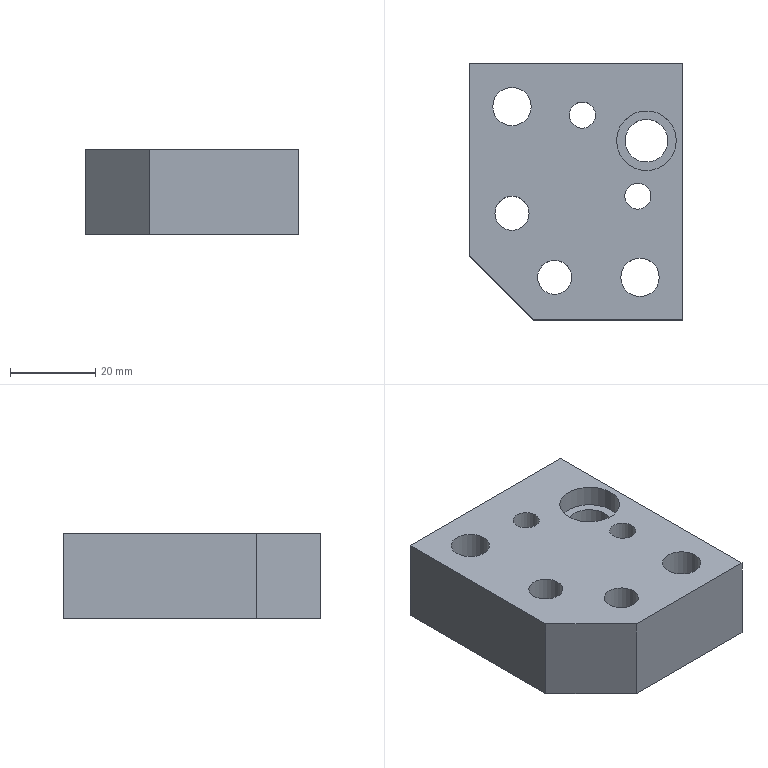Part | STEP file | 420_id2486_x_t | 1 solid | 24 faces | box 50 x 60 x 20 mm | volume 47706 mm3 | plane 12 | cylinder 12 | commonest cylinder face diameters 10 x3 14 x3 6.1 x2 8 x2 9 x2